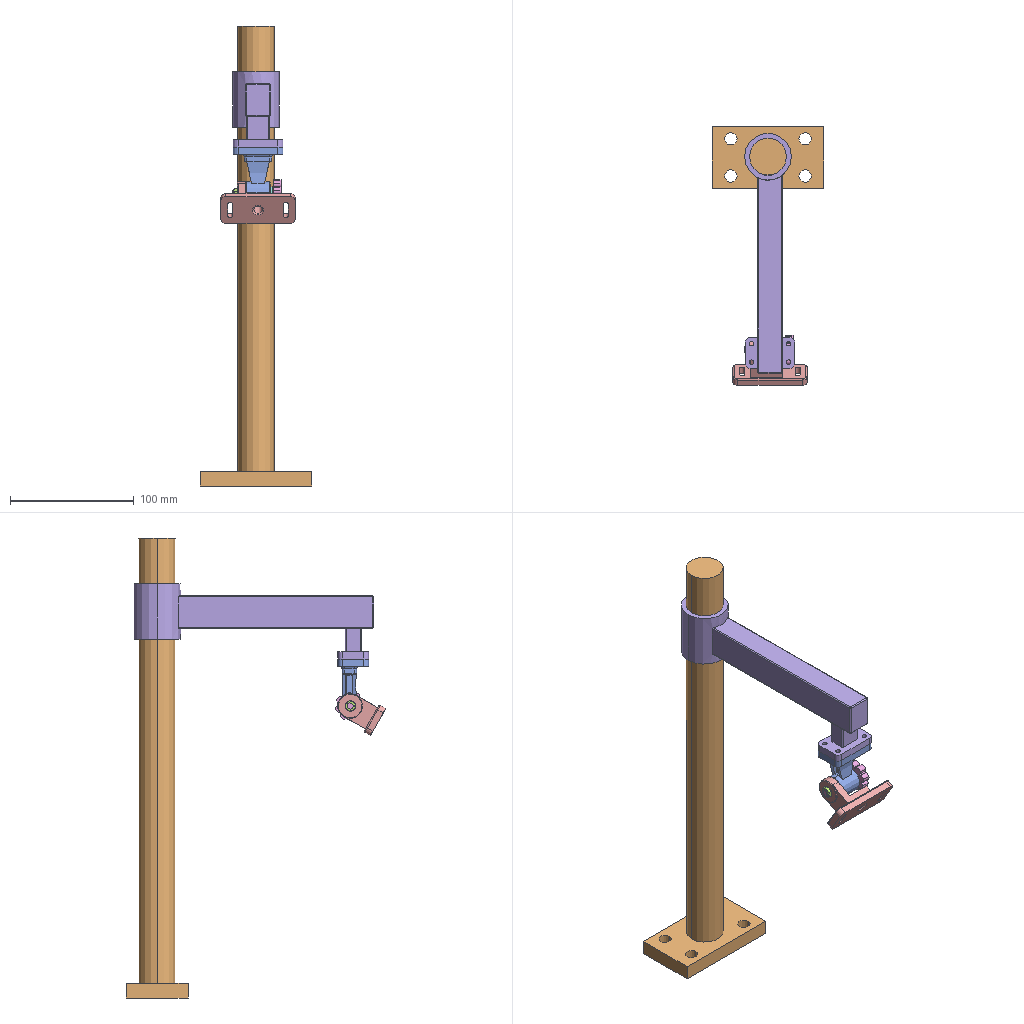Assembly | SolidWorks | 7 different items | 7 placed | box 90 x 210 x 372 mm
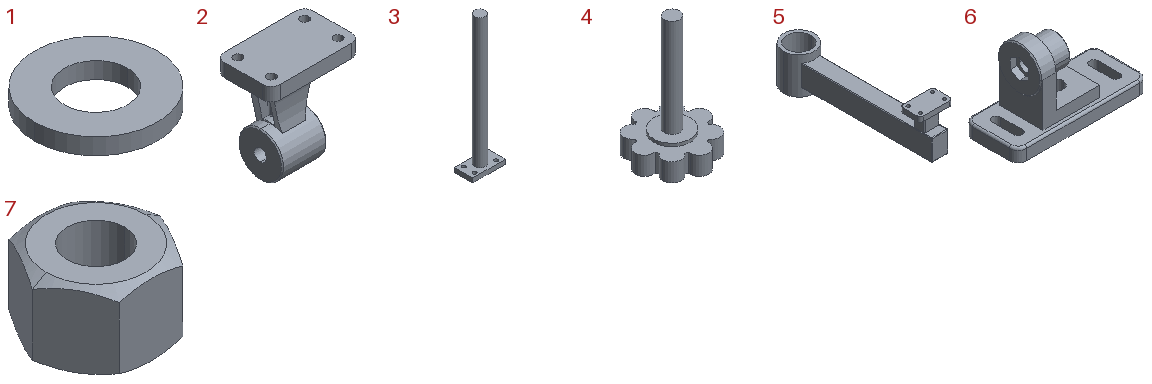Parts list (item | quantity | size | volume | features):
1 | x1 | 12 x 12 x 1.6 mm | 132.962 mm3 | features Extrusion 1
2 | x1 | 40 x 25 x 48 mm | 13548 mm3 | features ICE 8, Fillet 3, Chamfer 2, Extrusion 1
3 | x1 | 90 x 50 x 372 mm | 304699 mm3 | features Extrusion 1, ICE 1
4 | x1 | 24 x 24 x 39 mm | 2986 mm3 | features ICE 3, Extrusion 1
5 | x1 | 40.662 x 194 x 61 mm | 110850 mm3 | features ICE 3, Extrusion 1, Fillet 1
6 | x1 | 60 x 25 x 36 mm | 14469 mm3 | features ICE 6, Chamfer 3, Extrusion 1, Fillet 1
7 | x1 | 9.238 x 8 x 5.6 mm | 229.89 mm3 | features RevCut 2, Extrusion 1, LPattern 1
Mates (type | each side: item.copy, entity, surface, feature):
Concentric | 6.1 face cylinder Cut-Extrude1 | 2.1 face cylinder Cut-Extrude5
Coincident | 6.1 face plane Boss-Extrude2 | 2.1 face plane Boss-Extrude4
Coincident | 6.1 face plane Cut-Extrude2 | 7.1 face plane BaseNut
Concentric | 6.1 face cylinder Cut-Extrude1 | 7.1 face cylinder BaseNut
Concentric | 2.1 face cylinder Cut-Extrude5 | 4.1 face cylinder Boss-Extrude2
Parallel | 6.1 face plane Cut-Extrude2 | 7.1 face plane BaseNut
Coincident | 2.1 face plane Boss-Extrude4 | 1.1 face plane Base-Extrude
Concentric | 4.1 face cylinder Boss-Extrude2 | 1.1 face cylinder Base-Extrude
Coincident | 4.1 face plane Boss-Extrude3 | 1.1 face plane Base-Extrude
Concentric | 3.1 face cylinder Boss-Extrude2 | 5.1 face cylinder Boss-Extrude4
Coincident | 2.1 face plane Boss-Extrude1 | 5.1 face plane Boss-Extrude1 | 3 times
Parallel | 3.1 face plane Boss-Extrude1 | 5.1 face plane Boss-Extrude3
Coincident | 3.1 face plane Boss-Extrude1 | assembly plane | 2 times